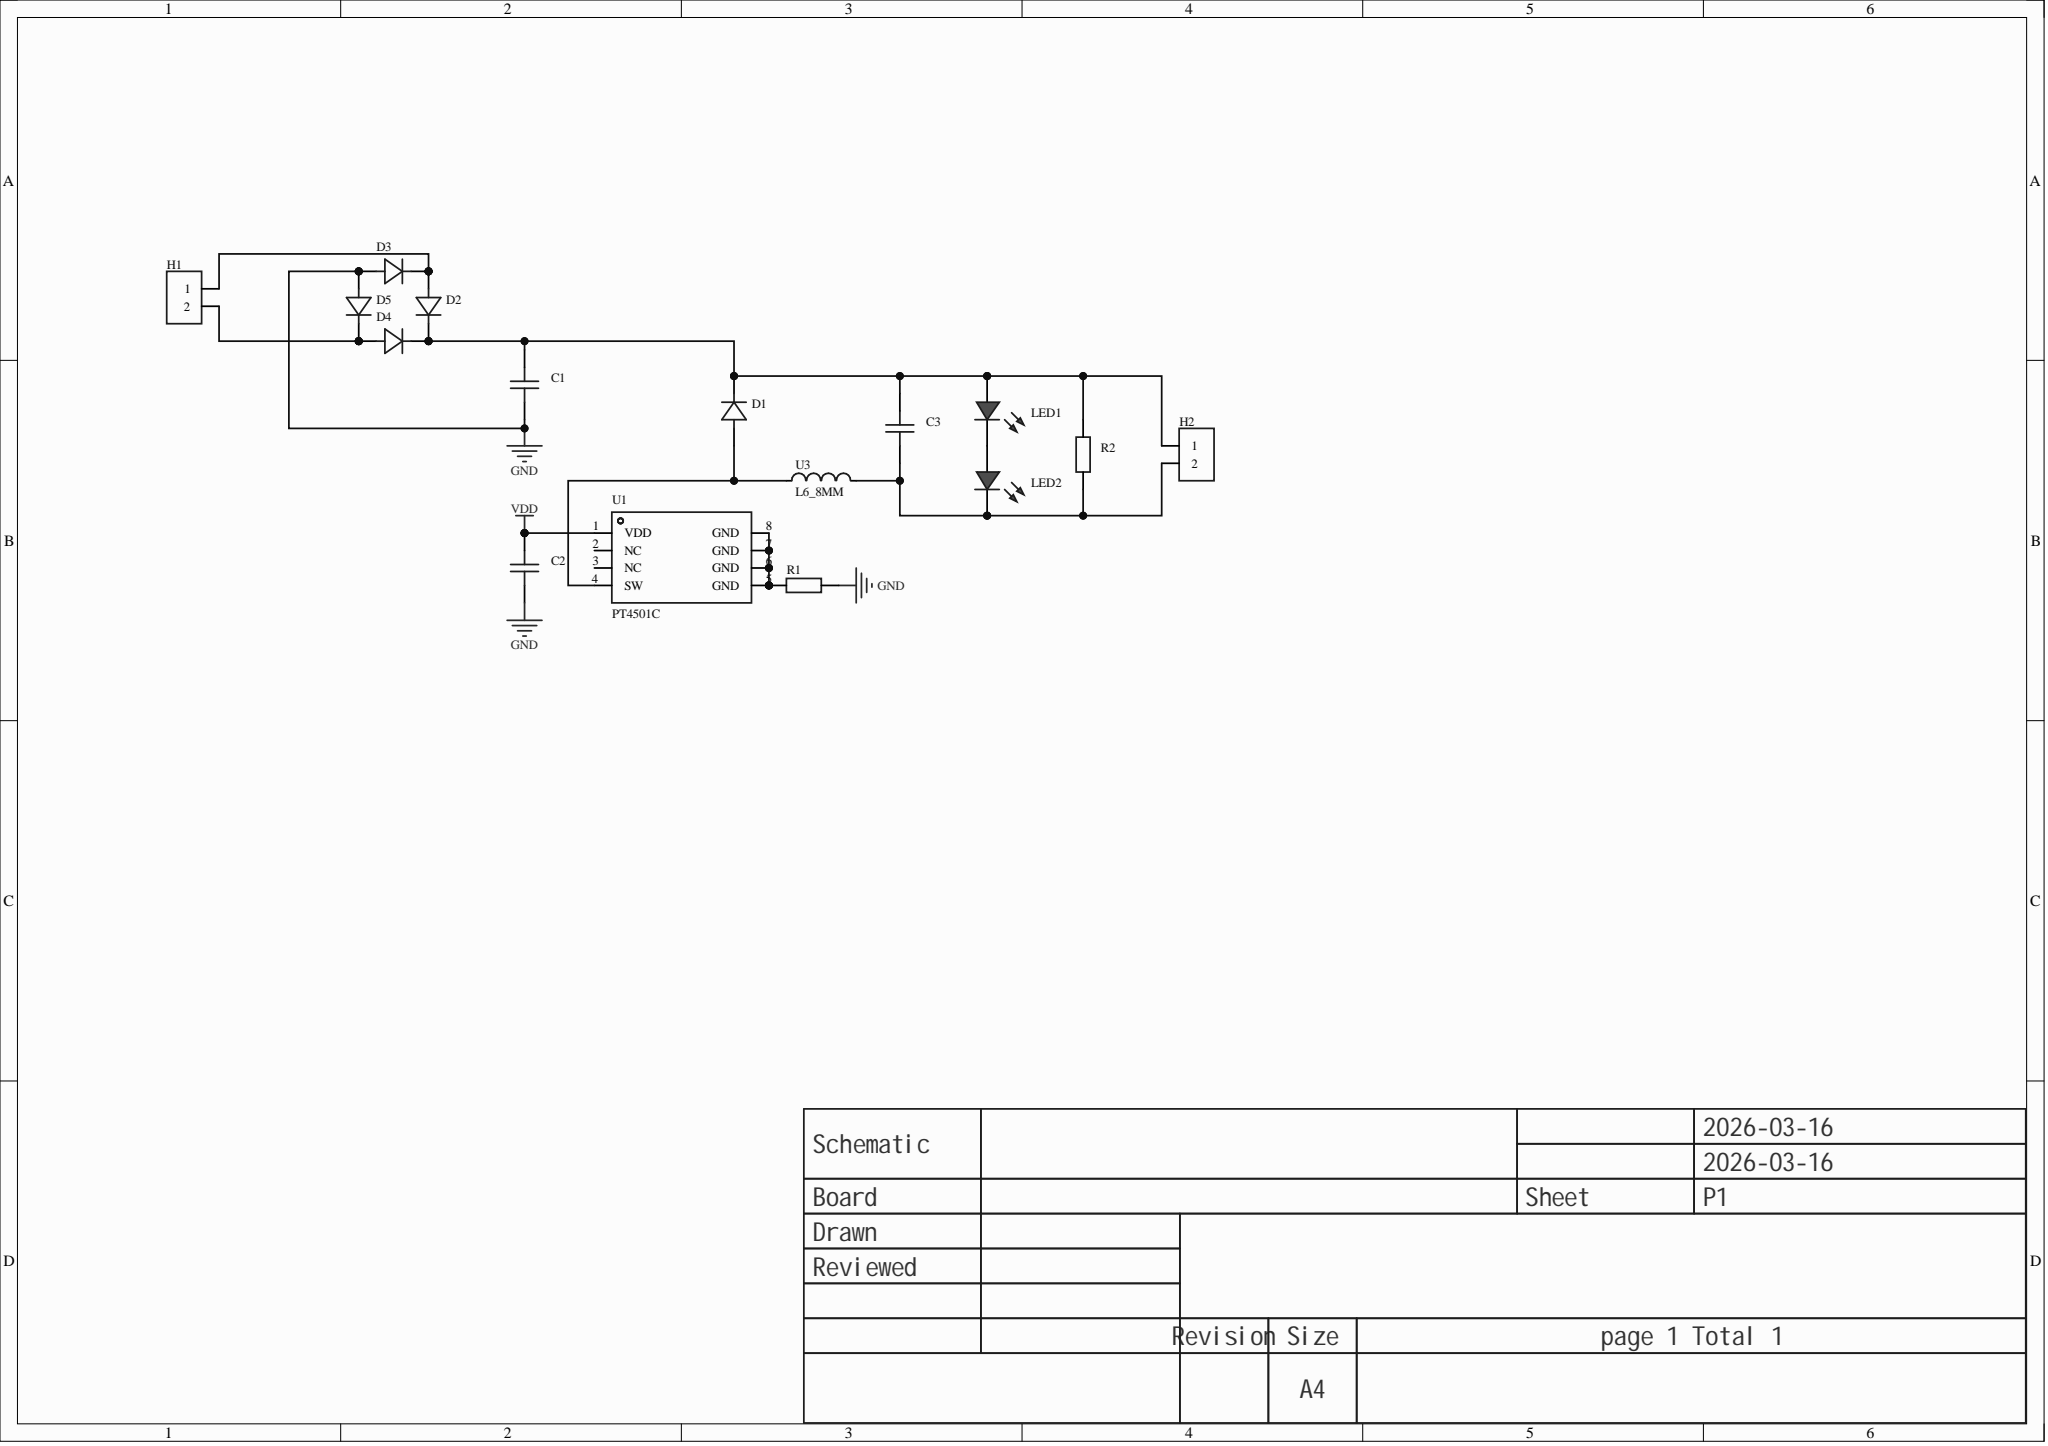Circuit board | Altium Designer | 16 parts | 9 nets
Bill of materials:
Comment,Description,Designator,Footprint,LibRef,Quantity
"100nF","","C1, C2, C3","CAP-TH_L5.0-W2.5-P5.00-D1.0","100nF","3"
"","","D1, D2, D3, D4, D5","DO_1N4007","D_1N4007A","5"
"","","H1, H2","HDR-TH_2P-P2.54-V-F","HDR-F_2.54_1x2P","2"
"","","LED1, LED2","LED_TH-3mm","LED_TH-R_3mm","2"
"10kO","","R1, R2","Res_1/2W","Res_AXIAL-1/2W","2"
"PT4501C","component PT4501C componentd Dual-channel single-stage linear LED driver IC","U1","SOP-8_L4.9-W3.9-P1.27-LS6.0-BL-EP","PT4501C","1"
"L6_8MM","","U3","IND-TH_BD6.00-P3.00-D0.6","L6_8MM","1"
Netlist (Protel format):
[
C1
CAP-TH_L5.0-W2.5-P5.00-D1.0
100nF



]
[
C2
CAP-TH_L5.0-W2.5-P5.00-D1.0
100nF



]
[
C3
CAP-TH_L5.0-W2.5-P5.00-D1.0
100nF



]
[
D1
DO_1N4007




]
[
D2
DO_1N4007




]
[
D3
DO_1N4007




]
[
D4
DO_1N4007




]
[
D5
DO_1N4007




]
[
H1
HDR-TH_2P-P2.54-V-F




]
[
H2
HDR-TH_2P-P2.54-V-F




]
[
LED1
LED_TH-3mm




]
[
LED2
LED_TH-3mm




]
[
R1
Res_1/2W
10kO



]
[
R2
Res_1/2W
10kO



]
[
U1
SOP-8_L4.9-W3.9-P1.27-LS6.0-BL-EP
PT4501C



]
[
U3
IND-TH_BD6.00-P3.00-D0.6
L6_8MM



]
(
VDD
C2-1
U1-1
)
(
NetR1_1
R1-1
U1-5
U1-6
U1-7
U1-8
)
(
NetLED1_2
LED1-2
LED2-1
)
(
NetD4_2
D4-2
D5-1
H1-2
)
(
NetD2_2
D2-2
D3-1
H1-1
)
(
NetD1_2
D1-2
U1-4
U3-1
)
(
NetC3_2
C3-2
H2-2
LED2-2
R2-1
U3-2
)
(
NetC1_1
C1-1
C3-1
D1-1
D2-1
D4-1
H2-1
LED1-1
R2-2
)
(
GND
C1-2
C2-2
D3-2
D5-2
R1-2
)